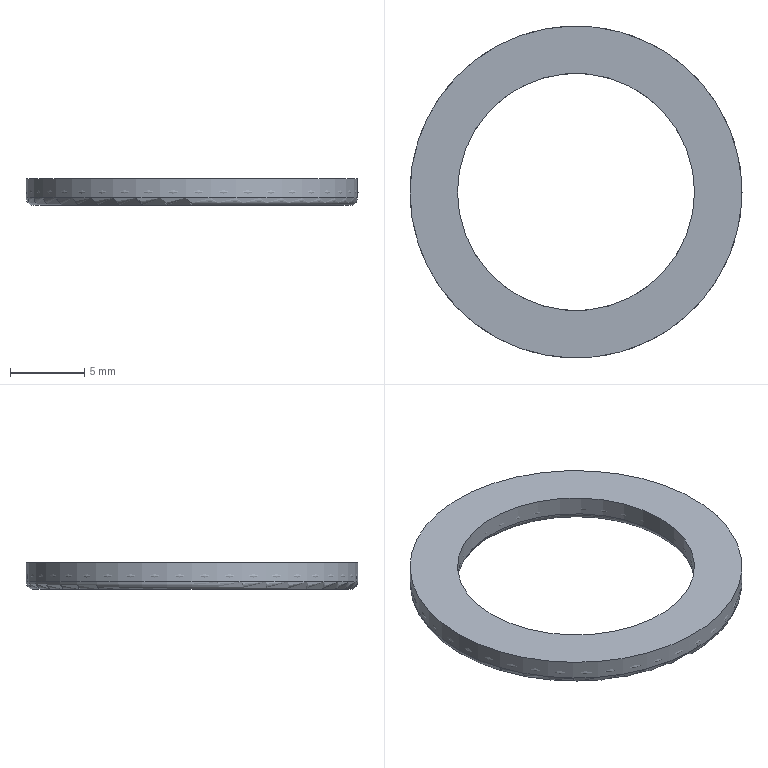Part | STEP file | EC21600001 | 2 solids | 7 faces | box 22.4 x 22.4 x 1.8 mm | volume 613.838 mm3 | cylinder 2 | plane 2 | torus 2 | other 1 | commonest cylinder face diameters 16 x1 22.4 x1
STEP:
#1=CARTESIAN_POINT('',(0.,0.,0.));
#2=DIRECTION('',(0.,0.,1.));
#3=DIRECTION('',(1.,0.,0.));
#4=AXIS2_PLACEMENT_3D('',#1,#2,#3);
#5=CARTESIAN_POINT('',(11.2,0.,-0.9));
#6=VERTEX_POINT('',#5);
#7=CARTESIAN_POINT('',(9.6,0.,-0.9));
#8=DIRECTION('',(0.,-1.,0.));
#9=DIRECTION('',(1.,0.,0.));
#10=AXIS2_PLACEMENT_3D('',#7,#8,#9);
#11=ELLIPSE('',#10,1.6,0.9);
#12=CARTESIAN_POINT('',(9.6,0.,-0.9));
#13=DIRECTION('',(0.,-1.,0.));
#14=DIRECTION('',(1.,0.,0.));
#15=AXIS2_PLACEMENT_3D('',#12,#13,#14);
#16=ELLIPSE('',#15,1.6,0.9);
#17=CARTESIAN_POINT('',(0.,0.,0.));
#18=DIRECTION('',(0.,0.,-1.));
#19=AXIS1_PLACEMENT('',#17,#18);
#20=SURFACE_OF_REVOLUTION('',#16,#19);
#21=CARTESIAN_POINT('',(0.,0.));
#22=DIRECTION('',(0.,1.));
#23=VECTOR('',#22,1.);
#24=LINE('',#21,#23);
#25=(GEOMETRIC_REPRESENTATION_CONTEXT(2)PARAMETRIC_REPRESENTATION_CONTEXT()REPRESENTATION_CONTEXT('',''));
#26=DEFINITIONAL_REPRESENTATION('',(#24),#25);
#27=PCURVE('',#20,#26);
#28=CARTESIAN_POINT('',(6.283,0.));
#29=DIRECTION('',(0.,1.));
#30=VECTOR('',#29,1.);
#31=LINE('',#28,#30);
#32=(GEOMETRIC_REPRESENTATION_CONTEXT(2)PARAMETRIC_REPRESENTATION_CONTEXT()REPRESENTATION_CONTEXT('',''));
#33=DEFINITIONAL_REPRESENTATION('',(#31),#32);
#34=PCURVE('',#20,#33);
#35=SEAM_CURVE('',#11,(#27,#34),.PCURVE_S1.);
#36=EDGE_CURVE('',#6,#6,#35,.T.);
#37=ORIENTED_EDGE('',*,*,#36,.F.);
#38=CARTESIAN_POINT('',(0.,0.,-0.9));
#39=DIRECTION('',(0.,0.,-1.));
#40=DIRECTION('',(1.,0.,0.));
#41=AXIS2_PLACEMENT_3D('',#38,#39,#40);
#42=CIRCLE('',#41,11.2);
#43=CARTESIAN_POINT('',(0.,0.));
#44=DIRECTION('',(1.,0.));
#45=VECTOR('',#44,1.);
#46=LINE('',#43,#45);
#47=(GEOMETRIC_REPRESENTATION_CONTEXT(2)PARAMETRIC_REPRESENTATION_CONTEXT()REPRESENTATION_CONTEXT('',''));
#48=DEFINITIONAL_REPRESENTATION('',(#46),#47);
#49=PCURVE('',#20,#48);
#50=CARTESIAN_POINT('',(0.,6.283));
#51=DIRECTION('',(1.,0.));
#52=VECTOR('',#51,1.);
#53=LINE('',#50,#52);
#54=(GEOMETRIC_REPRESENTATION_CONTEXT(2)PARAMETRIC_REPRESENTATION_CONTEXT()REPRESENTATION_CONTEXT('',''));
#55=DEFINITIONAL_REPRESENTATION('',(#53),#54);
#56=PCURVE('',#20,#55);
#57=SEAM_CURVE('',#42,(#49,#56),.PCURVE_S1.);
#58=EDGE_CURVE('',#6,#6,#57,.T.);
#59=ORIENTED_EDGE('',*,*,#58,.T.);
#60=ORIENTED_EDGE('',*,*,#36,.T.);
#61=ORIENTED_EDGE('',*,*,#58,.F.);
#62=EDGE_LOOP('',(#37,#59,#60,#61));
#63=FACE_BOUND('',#62,.F.);
#64=ADVANCED_FACE('',(#63),#20,.F.);
#65=CLOSED_SHELL('',(#64));
#66=MANIFOLD_SOLID_BREP('',#65);
#67=CARTESIAN_POINT('',(-11.2,0.,-1.3));
#68=VERTEX_POINT('',#67);
#69=CARTESIAN_POINT('',(0.,0.,-1.3));
#70=DIRECTION('',(0.,0.,1.));
#71=DIRECTION('',(-1.,0.,0.));
#72=AXIS2_PLACEMENT_3D('',#69,#70,#71);
#73=CIRCLE('',#72,11.2);
#74=CARTESIAN_POINT('',(0.,0.,-1.4));
#75=DIRECTION('',(0.,0.,1.));
#76=DIRECTION('',(1.,0.,0.));
#77=AXIS2_PLACEMENT_3D('',#74,#75,#76);
#78=CYLINDRICAL_SURFACE('',#77,11.2);
#79=CARTESIAN_POINT('',(3.142,0.1));
#80=DIRECTION('',(1.,0.));
#81=VECTOR('',#80,1.);
#82=LINE('',#79,#81);
#83=(GEOMETRIC_REPRESENTATION_CONTEXT(2)PARAMETRIC_REPRESENTATION_CONTEXT()REPRESENTATION_CONTEXT('',''));
#84=DEFINITIONAL_REPRESENTATION('',(#82),#83);
#85=PCURVE('',#78,#84);
#86=CARTESIAN_POINT('',(0.,0.,-1.3));
#87=DIRECTION('',(0.,0.,-1.));
#88=DIRECTION('',(-1.,0.,0.));
#89=AXIS2_PLACEMENT_3D('',#86,#87,#88);
#90=TOROIDAL_SURFACE('',#89,10.7,0.5);
#91=CARTESIAN_POINT('',(6.283,6.283));
#92=DIRECTION('',(-1.,0.));
#93=VECTOR('',#92,1.);
#94=LINE('',#91,#93);
#95=(GEOMETRIC_REPRESENTATION_CONTEXT(2)PARAMETRIC_REPRESENTATION_CONTEXT()REPRESENTATION_CONTEXT('',''));
#96=DEFINITIONAL_REPRESENTATION('',(#94),#95);
#97=PCURVE('',#90,#96);
#98=SURFACE_CURVE('',#73,(#85,#97),.PCURVE_S1.);
#99=EDGE_CURVE('',#68,#68,#98,.T.);
#100=ORIENTED_EDGE('',*,*,#99,.T.);
#101=CARTESIAN_POINT('',(-11.2,0.,0.));
#102=VERTEX_POINT('',#101);
#103=CARTESIAN_POINT('',(-11.2,0.,-1.3));
#104=CARTESIAN_POINT('',(-11.2,0.,0.));
#105=B_SPLINE_CURVE_WITH_KNOTS('',1,(#103,#104),.UNSPECIFIED.,.F.,.F.,(2,2),(0.1,1.4),.PIECEWISE_BEZIER_KNOTS.);
#106=CARTESIAN_POINT('',(9.425,0.));
#107=DIRECTION('',(0.,1.));
#108=VECTOR('',#107,1.);
#109=LINE('',#106,#108);
#110=(GEOMETRIC_REPRESENTATION_CONTEXT(2)PARAMETRIC_REPRESENTATION_CONTEXT()REPRESENTATION_CONTEXT('',''));
#111=DEFINITIONAL_REPRESENTATION('',(#109),#110);
#112=PCURVE('',#78,#111);
#113=CARTESIAN_POINT('',(3.142,0.));
#114=DIRECTION('',(0.,1.));
#115=VECTOR('',#114,1.);
#116=LINE('',#113,#115);
#117=(GEOMETRIC_REPRESENTATION_CONTEXT(2)PARAMETRIC_REPRESENTATION_CONTEXT()REPRESENTATION_CONTEXT('',''));
#118=DEFINITIONAL_REPRESENTATION('',(#116),#117);
#119=PCURVE('',#78,#118);
#120=SEAM_CURVE('',#105,(#112,#119),.PCURVE_S1.);
#121=EDGE_CURVE('',#68,#102,#120,.T.);
#122=ORIENTED_EDGE('',*,*,#121,.T.);
#123=CARTESIAN_POINT('',(0.,0.,0.));
#124=DIRECTION('',(0.,0.,-1.));
#125=DIRECTION('',(-1.,0.,0.));
#126=AXIS2_PLACEMENT_3D('',#123,#124,#125);
#127=CIRCLE('',#126,11.2);
#128=CARTESIAN_POINT('',(9.425,1.4));
#129=DIRECTION('',(-1.,0.));
#130=VECTOR('',#129,1.);
#131=LINE('',#128,#130);
#132=(GEOMETRIC_REPRESENTATION_CONTEXT(2)PARAMETRIC_REPRESENTATION_CONTEXT()REPRESENTATION_CONTEXT('',''));
#133=DEFINITIONAL_REPRESENTATION('',(#131),#132);
#134=PCURVE('',#78,#133);
#135=CARTESIAN_POINT('',(0.,0.,0.));
#136=DIRECTION('',(0.,0.,-1.));
#137=DIRECTION('',(-1.,0.,0.));
#138=AXIS2_PLACEMENT_3D('',#135,#136,#137);
#139=PLANE('',#138);
#140=CARTESIAN_POINT('',(0.,0.));
#141=DIRECTION('',(1.,0.));
#142=AXIS2_PLACEMENT_2D('',#140,#141);
#143=CIRCLE('',#142,11.2);
#144=(GEOMETRIC_REPRESENTATION_CONTEXT(2)PARAMETRIC_REPRESENTATION_CONTEXT()REPRESENTATION_CONTEXT('',''));
#145=DEFINITIONAL_REPRESENTATION('',(#143),#144);
#146=PCURVE('',#139,#145);
#147=SURFACE_CURVE('',#127,(#134,#146),.PCURVE_S1.);
#148=EDGE_CURVE('',#102,#102,#147,.T.);
#149=ORIENTED_EDGE('',*,*,#148,.T.);
#150=ORIENTED_EDGE('',*,*,#121,.F.);
#151=EDGE_LOOP('',(#100,#122,#149,#150));
#152=FACE_BOUND('',#151,.T.);
#153=ADVANCED_FACE('',(#152),#78,.T.);
#154=CARTESIAN_POINT('',(-8.,0.,-1.3));
#155=VERTEX_POINT('',#154);
#156=CARTESIAN_POINT('',(0.,0.,-1.3));
#157=DIRECTION('',(0.,0.,-1.));
#158=DIRECTION('',(-1.,0.,0.));
#159=AXIS2_PLACEMENT_3D('',#156,#157,#158);
#160=CIRCLE('',#159,8.);
#161=CARTESIAN_POINT('',(0.,0.,-1.4));
#162=DIRECTION('',(0.,0.,1.));
#163=DIRECTION('',(1.,0.,0.));
#164=AXIS2_PLACEMENT_3D('',#161,#162,#163);
#165=CYLINDRICAL_SURFACE('',#164,8.);
#166=CARTESIAN_POINT('',(9.425,0.1));
#167=DIRECTION('',(-1.,0.));
#168=VECTOR('',#167,1.);
#169=LINE('',#166,#168);
#170=(GEOMETRIC_REPRESENTATION_CONTEXT(2)PARAMETRIC_REPRESENTATION_CONTEXT()REPRESENTATION_CONTEXT('',''));
#171=DEFINITIONAL_REPRESENTATION('',(#169),#170);
#172=PCURVE('',#165,#171);
#173=CARTESIAN_POINT('',(0.,0.,-1.3));
#174=DIRECTION('',(0.,0.,-1.));
#175=DIRECTION('',(-1.,0.,0.));
#176=AXIS2_PLACEMENT_3D('',#173,#174,#175);
#177=TOROIDAL_SURFACE('',#176,8.5,0.5);
#178=CARTESIAN_POINT('',(0.,9.425));
#179=DIRECTION('',(1.,0.));
#180=VECTOR('',#179,1.);
#181=LINE('',#178,#180);
#182=(GEOMETRIC_REPRESENTATION_CONTEXT(2)PARAMETRIC_REPRESENTATION_CONTEXT()REPRESENTATION_CONTEXT('',''));
#183=DEFINITIONAL_REPRESENTATION('',(#181),#182);
#184=PCURVE('',#177,#183);
#185=SURFACE_CURVE('',#160,(#172,#184),.PCURVE_S1.);
#186=EDGE_CURVE('',#155,#155,#185,.T.);
#187=ORIENTED_EDGE('',*,*,#186,.F.);
#188=CARTESIAN_POINT('',(-8.,0.,0.));
#189=VERTEX_POINT('',#188);
#190=CARTESIAN_POINT('',(-8.,0.,-1.3));
#191=CARTESIAN_POINT('',(-8.,0.,0.));
#192=B_SPLINE_CURVE_WITH_KNOTS('',1,(#190,#191),.UNSPECIFIED.,.F.,.F.,(2,2),(0.1,1.4),.PIECEWISE_BEZIER_KNOTS.);
#193=CARTESIAN_POINT('',(9.425,0.));
#194=DIRECTION('',(0.,1.));
#195=VECTOR('',#194,1.);
#196=LINE('',#193,#195);
#197=(GEOMETRIC_REPRESENTATION_CONTEXT(2)PARAMETRIC_REPRESENTATION_CONTEXT()REPRESENTATION_CONTEXT('',''));
#198=DEFINITIONAL_REPRESENTATION('',(#196),#197);
#199=PCURVE('',#165,#198);
#200=CARTESIAN_POINT('',(3.142,0.));
#201=DIRECTION('',(0.,1.));
#202=VECTOR('',#201,1.);
#203=LINE('',#200,#202);
#204=(GEOMETRIC_REPRESENTATION_CONTEXT(2)PARAMETRIC_REPRESENTATION_CONTEXT()REPRESENTATION_CONTEXT('',''));
#205=DEFINITIONAL_REPRESENTATION('',(#203),#204);
#206=PCURVE('',#165,#205);
#207=SEAM_CURVE('',#192,(#199,#206),.PCURVE_S1.);
#208=EDGE_CURVE('',#155,#189,#207,.T.);
#209=ORIENTED_EDGE('',*,*,#208,.T.);
#210=CARTESIAN_POINT('',(0.,0.,0.));
#211=DIRECTION('',(0.,0.,-1.));
#212=DIRECTION('',(-1.,0.,0.));
#213=AXIS2_PLACEMENT_3D('',#210,#211,#212);
#214=CIRCLE('',#213,8.);
#215=CARTESIAN_POINT('',(9.425,1.4));
#216=DIRECTION('',(-1.,0.));
#217=VECTOR('',#216,1.);
#218=LINE('',#215,#217);
#219=(GEOMETRIC_REPRESENTATION_CONTEXT(2)PARAMETRIC_REPRESENTATION_CONTEXT()REPRESENTATION_CONTEXT('',''));
#220=DEFINITIONAL_REPRESENTATION('',(#218),#219);
#221=PCURVE('',#165,#220);
#222=CARTESIAN_POINT('',(0.,0.));
#223=DIRECTION('',(1.,0.));
#224=AXIS2_PLACEMENT_2D('',#222,#223);
#225=CIRCLE('',#224,8.);
#226=(GEOMETRIC_REPRESENTATION_CONTEXT(2)PARAMETRIC_REPRESENTATION_CONTEXT()REPRESENTATION_CONTEXT('',''));
#227=DEFINITIONAL_REPRESENTATION('',(#225),#226);
#228=PCURVE('',#139,#227);
#229=SURFACE_CURVE('',#214,(#221,#228),.PCURVE_S1.);
#230=EDGE_CURVE('',#189,#189,#229,.T.);
#231=ORIENTED_EDGE('',*,*,#230,.T.);
#232=ORIENTED_EDGE('',*,*,#208,.F.);
#233=EDGE_LOOP('',(#187,#209,#231,#232));
#234=FACE_BOUND('',#233,.F.);
#235=ADVANCED_FACE('',(#234),#165,.F.);
#236=CARTESIAN_POINT('',(-10.7,0.,-1.8));
#237=VERTEX_POINT('',#236);
#238=CARTESIAN_POINT('',(0.,0.,-1.8));
#239=DIRECTION('',(0.,0.,-1.));
#240=DIRECTION('',(-1.,0.,0.));
#241=AXIS2_PLACEMENT_3D('',#238,#239,#240);
#242=CIRCLE('',#241,10.7);
#243=CARTESIAN_POINT('',(0.,0.,-1.8));
#244=DIRECTION('',(0.,0.,-1.));
#245=DIRECTION('',(-1.,0.,0.));
#246=AXIS2_PLACEMENT_3D('',#243,#244,#245);
#247=PLANE('',#246);
#248=CARTESIAN_POINT('',(0.,0.));
#249=DIRECTION('',(1.,0.));
#250=AXIS2_PLACEMENT_2D('',#248,#249);
#251=CIRCLE('',#250,10.7);
#252=(GEOMETRIC_REPRESENTATION_CONTEXT(2)PARAMETRIC_REPRESENTATION_CONTEXT()REPRESENTATION_CONTEXT('',''));
#253=DEFINITIONAL_REPRESENTATION('',(#251),#252);
#254=PCURVE('',#247,#253);
#255=CARTESIAN_POINT('',(0.,7.854));
#256=DIRECTION('',(1.,0.));
#257=VECTOR('',#256,1.);
#258=LINE('',#255,#257);
#259=(GEOMETRIC_REPRESENTATION_CONTEXT(2)PARAMETRIC_REPRESENTATION_CONTEXT()REPRESENTATION_CONTEXT('',''));
#260=DEFINITIONAL_REPRESENTATION('',(#258),#259);
#261=PCURVE('',#90,#260);
#262=SURFACE_CURVE('',#242,(#254,#261),.PCURVE_S1.);
#263=EDGE_CURVE('',#237,#237,#262,.T.);
#264=ORIENTED_EDGE('',*,*,#263,.T.);
#265=EDGE_LOOP('',(#264));
#266=FACE_BOUND('',#265,.T.);
#267=CARTESIAN_POINT('',(-8.5,0.,-1.8));
#268=VERTEX_POINT('',#267);
#269=CARTESIAN_POINT('',(0.,0.,-1.8));
#270=DIRECTION('',(0.,0.,1.));
#271=DIRECTION('',(-1.,0.,0.));
#272=AXIS2_PLACEMENT_3D('',#269,#270,#271);
#273=CIRCLE('',#272,8.5);
#274=CARTESIAN_POINT('',(8.5,0.));
#275=CARTESIAN_POINT('',(8.5,-14.722));
#276=CARTESIAN_POINT('',(-4.25,-7.361));
#277=CARTESIAN_POINT('',(-17.,0.));
#278=CARTESIAN_POINT('',(-4.25,7.361));
#279=CARTESIAN_POINT('',(8.5,14.722));
#280=CARTESIAN_POINT('',(8.5,0.));
#281=(BOUNDED_CURVE()B_SPLINE_CURVE(2,(#274,#275,#276,#277,#278,#279,#280),.UNSPECIFIED.,.T.,.F.)B_SPLINE_CURVE_WITH_KNOTS((1,2,2,2,2,1),(-2.094,0.,2.094,4.189,6.283,8.378),.UNSPECIFIED.)CURVE()GEOMETRIC_REPRESENTATION_ITEM()RATIONAL_B_SPLINE_CURVE((1.,0.5,1.,0.5,1.,0.5,1.))REPRESENTATION_ITEM(''));
#282=(GEOMETRIC_REPRESENTATION_CONTEXT(2)PARAMETRIC_REPRESENTATION_CONTEXT()REPRESENTATION_CONTEXT('',''));
#283=DEFINITIONAL_REPRESENTATION('',(#281),#282);
#284=PCURVE('',#247,#283);
#285=CARTESIAN_POINT('',(6.283,7.854));
#286=DIRECTION('',(-1.,0.));
#287=VECTOR('',#286,1.);
#288=LINE('',#285,#287);
#289=(GEOMETRIC_REPRESENTATION_CONTEXT(2)PARAMETRIC_REPRESENTATION_CONTEXT()REPRESENTATION_CONTEXT('',''));
#290=DEFINITIONAL_REPRESENTATION('',(#288),#289);
#291=PCURVE('',#177,#290);
#292=SURFACE_CURVE('',#273,(#284,#291),.PCURVE_S1.);
#293=EDGE_CURVE('',#268,#268,#292,.T.);
#294=ORIENTED_EDGE('',*,*,#293,.T.);
#295=EDGE_LOOP('',(#294));
#296=FACE_BOUND('',#295,.T.);
#297=ADVANCED_FACE('',(#266,#296),#247,.T.);
#298=ORIENTED_EDGE('',*,*,#148,.F.);
#299=EDGE_LOOP('',(#298));
#300=FACE_BOUND('',#299,.T.);
#301=ORIENTED_EDGE('',*,*,#230,.T.);
#302=EDGE_LOOP('',(#301));
#303=FACE_BOUND('',#302,.T.);
#304=ADVANCED_FACE('',(#300,#303),#139,.F.);
#305=ORIENTED_EDGE('',*,*,#263,.F.);
#306=CARTESIAN_POINT('',(-11.2,0.,-1.3));
#307=CARTESIAN_POINT('',(-11.2,0.,-1.434));
#308=CARTESIAN_POINT('',(-11.157,0.,-1.564));
#309=CARTESIAN_POINT('',(-11.076,0.,-1.676));
#310=CARTESIAN_POINT('',(-10.964,0.,-1.757));
#311=CARTESIAN_POINT('',(-10.834,0.,-1.8));
#312=CARTESIAN_POINT('',(-10.7,0.,-1.8));
#313=(BOUNDED_CURVE()B_SPLINE_CURVE(6,(#306,#307,#308,#309,#310,#311,#312),.UNSPECIFIED.,.F.,.F.)B_SPLINE_CURVE_WITH_KNOTS((7,7),(0.,1.571),.PIECEWISE_BEZIER_KNOTS.)CURVE()GEOMETRIC_REPRESENTATION_ITEM()RATIONAL_B_SPLINE_CURVE((1.031,1.01,0.9979,0.994,0.9979,1.01,1.031))REPRESENTATION_ITEM(''));
#314=CARTESIAN_POINT('',(0.,6.283));
#315=DIRECTION('',(0.,1.));
#316=VECTOR('',#315,1.);
#317=LINE('',#314,#316);
#318=(GEOMETRIC_REPRESENTATION_CONTEXT(2)PARAMETRIC_REPRESENTATION_CONTEXT()REPRESENTATION_CONTEXT('',''));
#319=DEFINITIONAL_REPRESENTATION('',(#317),#318);
#320=PCURVE('',#90,#319);
#321=CARTESIAN_POINT('',(6.283,6.283));
#322=DIRECTION('',(0.,1.));
#323=VECTOR('',#322,1.);
#324=LINE('',#321,#323);
#325=(GEOMETRIC_REPRESENTATION_CONTEXT(2)PARAMETRIC_REPRESENTATION_CONTEXT()REPRESENTATION_CONTEXT('',''));
#326=DEFINITIONAL_REPRESENTATION('',(#324),#325);
#327=PCURVE('',#90,#326);
#328=SEAM_CURVE('',#313,(#320,#327),.PCURVE_S1.);
#329=EDGE_CURVE('',#68,#237,#328,.T.);
#330=ORIENTED_EDGE('',*,*,#329,.F.);
#331=ORIENTED_EDGE('',*,*,#99,.F.);
#332=ORIENTED_EDGE('',*,*,#329,.T.);
#333=EDGE_LOOP('',(#305,#330,#331,#332));
#334=FACE_BOUND('',#333,.T.);
#335=ADVANCED_FACE('',(#334),#90,.T.);
#336=ORIENTED_EDGE('',*,*,#293,.F.);
#337=CARTESIAN_POINT('',(-8.5,0.,-1.8));
#338=CARTESIAN_POINT('',(-8.366,0.,-1.8));
#339=CARTESIAN_POINT('',(-8.236,0.,-1.757));
#340=CARTESIAN_POINT('',(-8.124,0.,-1.676));
#341=CARTESIAN_POINT('',(-8.043,0.,-1.564));
#342=CARTESIAN_POINT('',(-8.,0.,-1.434));
#343=CARTESIAN_POINT('',(-8.,0.,-1.3));
#344=(BOUNDED_CURVE()B_SPLINE_CURVE(6,(#337,#338,#339,#340,#341,#342,#343),.UNSPECIFIED.,.F.,.F.)B_SPLINE_CURVE_WITH_KNOTS((7,7),(1.571,3.142),.PIECEWISE_BEZIER_KNOTS.)CURVE()GEOMETRIC_REPRESENTATION_ITEM()RATIONAL_B_SPLINE_CURVE((1.031,1.01,0.9979,0.994,0.9979,1.01,1.031))REPRESENTATION_ITEM(''));
#345=CARTESIAN_POINT('',(6.283,6.283));
#346=DIRECTION('',(0.,1.));
#347=VECTOR('',#346,1.);
#348=LINE('',#345,#347);
#349=(GEOMETRIC_REPRESENTATION_CONTEXT(2)PARAMETRIC_REPRESENTATION_CONTEXT()REPRESENTATION_CONTEXT('',''));
#350=DEFINITIONAL_REPRESENTATION('',(#348),#349);
#351=PCURVE('',#177,#350);
#352=CARTESIAN_POINT('',(0.,6.283));
#353=DIRECTION('',(0.,1.));
#354=VECTOR('',#353,1.);
#355=LINE('',#352,#354);
#356=(GEOMETRIC_REPRESENTATION_CONTEXT(2)PARAMETRIC_REPRESENTATION_CONTEXT()REPRESENTATION_CONTEXT('',''));
#357=DEFINITIONAL_REPRESENTATION('',(#355),#356);
#358=PCURVE('',#177,#357);
#359=SEAM_CURVE('',#344,(#351,#358),.PCURVE_S1.);
#360=EDGE_CURVE('',#268,#155,#359,.T.);
#361=ORIENTED_EDGE('',*,*,#360,.T.);
#362=ORIENTED_EDGE('',*,*,#186,.F.);
#363=ORIENTED_EDGE('',*,*,#360,.F.);
#364=EDGE_LOOP('',(#336,#361,#362,#363));
#365=FACE_BOUND('',#364,.T.);
#366=ADVANCED_FACE('',(#365),#177,.T.);
#367=CLOSED_SHELL('',(#153,#235,#297,#304,#335,#366));
#368=MANIFOLD_SOLID_BREP('',#367);
#369=(LENGTH_UNIT()NAMED_UNIT(*)SI_UNIT(.MILLI.,.METRE.));
#370=UNCERTAINTY_MEASURE_WITH_UNIT(LENGTH_MEASURE(0.000005),#369,'','');
#371=(NAMED_UNIT(*)PLANE_ANGLE_UNIT()SI_UNIT($,.RADIAN.));
#372=(NAMED_UNIT(*)SI_UNIT($,.STERADIAN.)SOLID_ANGLE_UNIT());
#373=(GEOMETRIC_REPRESENTATION_CONTEXT(3)GLOBAL_UNCERTAINTY_ASSIGNED_CONTEXT((#370))GLOBAL_UNIT_ASSIGNED_CONTEXT((#369,#371,#372))REPRESENTATION_CONTEXT('',''));
#374=SHAPE_REPRESENTATION('',(#4,#66,#368),#373);